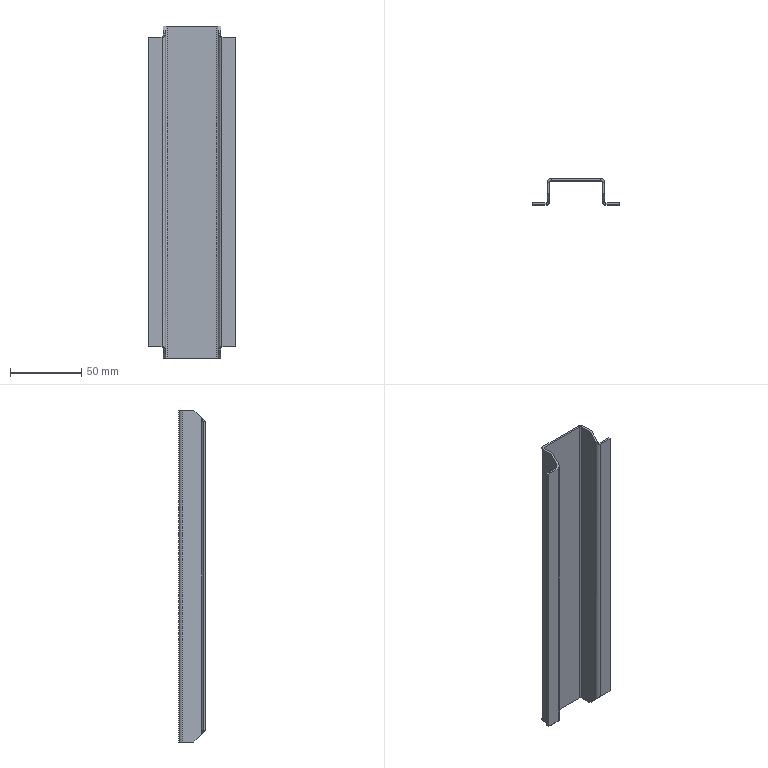Part | SolidWorks | features FlatPattern 1, ICE 1, SMBaseFlange 1, SheetMetal 1 | 1 solid | 42 faces | box 61 x 18.5 x 232.5 mm | volume 31420 mm3 | plane 30 | cylinder 8 | spline 4 | commonest cylinder face diameters 2 x4 5 x4
STEP:
#1=CARTESIAN_POINT('',(22.477,26.708,8.));
#2=VERTEX_POINT('',#1);
#3=CARTESIAN_POINT('',(12.977,26.708,8.));
#4=VERTEX_POINT('',#3);
#5=CARTESIAN_POINT('',(168.477,26.708,8.));
#6=DIRECTION('',(-1.,0.,0.));
#7=VECTOR('',#6,1000.);
#8=LINE('',#5,#7);
#9=EDGE_CURVE('',#2,#4,#8,.T.);
#10=ORIENTED_EDGE('',*,*,#9,.F.);
#11=CARTESIAN_POINT('',(22.477,26.708,224.5));
#12=VERTEX_POINT('',#11);
#13=CARTESIAN_POINT('',(22.477,26.708,232.5));
#14=DIRECTION('',(0.,0.,-1.));
#15=VECTOR('',#14,1000.);
#16=LINE('',#13,#15);
#17=EDGE_CURVE('',#12,#2,#16,.T.);
#18=ORIENTED_EDGE('',*,*,#17,.F.);
#19=CARTESIAN_POINT('',(12.977,26.708,224.5));
#20=VERTEX_POINT('',#19);
#21=CARTESIAN_POINT('',(168.477,26.708,224.5));
#22=DIRECTION('',(-1.,0.,0.));
#23=VECTOR('',#22,1000.);
#24=LINE('',#21,#23);
#25=EDGE_CURVE('',#12,#20,#24,.T.);
#26=ORIENTED_EDGE('',*,*,#25,.T.);
#27=CARTESIAN_POINT('',(12.977,26.708,232.5));
#28=DIRECTION('',(0.,0.,-1.));
#29=VECTOR('',#28,1000.);
#30=LINE('',#27,#29);
#31=EDGE_CURVE('',#20,#4,#30,.T.);
#32=ORIENTED_EDGE('',*,*,#31,.T.);
#33=EDGE_LOOP('',(#10,#18,#26,#32));
#34=FACE_OUTER_BOUND('',#33,.T.);
#35=CARTESIAN_POINT('',(11.977,26.708,232.5));
#36=DIRECTION('',(0.,1.,0.));
#37=DIRECTION('',(-1.,0.,0.));
#38=AXIS2_PLACEMENT_3D('',#35,#36,#37);
#39=PLANE('',#38);
#40=ADVANCED_FACE('',(#34),#39,.F.);
#41=ORIENTED_EDGE('',*,*,#17,.T.);
#42=CARTESIAN_POINT('',(22.477,28.208,8.));
#43=VERTEX_POINT('',#42);
#44=CARTESIAN_POINT('',(22.477,26.708,8.));
#45=DIRECTION('',(0.,1.,0.));
#46=VECTOR('',#45,1000.);
#47=LINE('',#44,#46);
#48=EDGE_CURVE('',#2,#43,#47,.T.);
#49=ORIENTED_EDGE('',*,*,#48,.T.);
#50=CARTESIAN_POINT('',(22.477,28.208,224.5));
#51=VERTEX_POINT('',#50);
#52=CARTESIAN_POINT('',(22.477,28.208,232.5));
#53=DIRECTION('',(0.,0.,-1.));
#54=VECTOR('',#53,1000.);
#55=LINE('',#52,#54);
#56=EDGE_CURVE('',#51,#43,#55,.T.);
#57=ORIENTED_EDGE('',*,*,#56,.F.);
#58=CARTESIAN_POINT('',(22.477,26.708,224.5));
#59=DIRECTION('',(0.,1.,0.));
#60=VECTOR('',#59,1000.);
#61=LINE('',#58,#60);
#62=EDGE_CURVE('',#12,#51,#61,.T.);
#63=ORIENTED_EDGE('',*,*,#62,.F.);
#64=EDGE_LOOP('',(#41,#49,#57,#63));
#65=FACE_OUTER_BOUND('',#64,.T.);
#66=CARTESIAN_POINT('',(22.477,28.208,232.5));
#67=DIRECTION('',(1.,0.,0.));
#68=DIRECTION('',(0.,0.,-1.));
#69=AXIS2_PLACEMENT_3D('',#66,#67,#68);
#70=PLANE('',#69);
#71=ADVANCED_FACE('',(#65),#70,.T.);
#72=ORIENTED_EDGE('',*,*,#56,.T.);
#73=CARTESIAN_POINT('',(12.977,28.208,8.));
#74=VERTEX_POINT('',#73);
#75=CARTESIAN_POINT('',(11.977,28.208,8.));
#76=DIRECTION('',(-1.,0.,0.));
#77=VECTOR('',#76,1000.);
#78=LINE('',#75,#77);
#79=EDGE_CURVE('',#43,#74,#78,.T.);
#80=ORIENTED_EDGE('',*,*,#79,.T.);
#81=CARTESIAN_POINT('',(12.977,28.208,224.5));
#82=VERTEX_POINT('',#81);
#83=CARTESIAN_POINT('',(12.977,28.208,232.5));
#84=DIRECTION('',(0.,0.,-1.));
#85=VECTOR('',#84,1000.);
#86=LINE('',#83,#85);
#87=EDGE_CURVE('',#82,#74,#86,.T.);
#88=ORIENTED_EDGE('',*,*,#87,.F.);
#89=CARTESIAN_POINT('',(11.977,28.208,224.5));
#90=DIRECTION('',(-1.,0.,0.));
#91=VECTOR('',#90,1000.);
#92=LINE('',#89,#91);
#93=EDGE_CURVE('',#51,#82,#92,.T.);
#94=ORIENTED_EDGE('',*,*,#93,.F.);
#95=EDGE_LOOP('',(#72,#80,#88,#94));
#96=FACE_OUTER_BOUND('',#95,.T.);
#97=CARTESIAN_POINT('',(11.977,28.208,232.5));
#98=DIRECTION('',(0.,1.,0.));
#99=DIRECTION('',(-1.,0.,0.));
#100=AXIS2_PLACEMENT_3D('',#97,#98,#99);
#101=PLANE('',#100);
#102=ADVANCED_FACE('',(#96),#101,.T.);
#103=ORIENTED_EDGE('',*,*,#87,.T.);
#104=CARTESIAN_POINT('',(11.977,29.208,5.5));
#105=VERTEX_POINT('',#104);
#106=CARTESIAN_POINT('',(11.977,29.208,5.5));
#107=CARTESIAN_POINT('',(11.977,28.623,6.964));
#108=CARTESIAN_POINT('',(12.391,28.208,8.));
#109=CARTESIAN_POINT('',(12.977,28.208,8.));
#110=(BOUNDED_CURVE()B_SPLINE_CURVE(3,(#106,#107,#108,#109),.UNSPECIFIED.,.F.,.F.)B_SPLINE_CURVE_WITH_KNOTS((4,4),(1.571,3.142),.UNSPECIFIED.)CURVE()GEOMETRIC_REPRESENTATION_ITEM()RATIONAL_B_SPLINE_CURVE((1.,0.8047,0.8047,1.))REPRESENTATION_ITEM(''));
#111=EDGE_CURVE('',#105,#74,#110,.T.);
#112=ORIENTED_EDGE('',*,*,#111,.F.);
#113=CARTESIAN_POINT('',(11.977,29.208,227.));
#114=VERTEX_POINT('',#113);
#115=CARTESIAN_POINT('',(11.977,29.208,232.5));
#116=DIRECTION('',(0.,0.,-1.));
#117=VECTOR('',#116,1000.);
#118=LINE('',#115,#117);
#119=EDGE_CURVE('',#114,#105,#118,.T.);
#120=ORIENTED_EDGE('',*,*,#119,.F.);
#121=CARTESIAN_POINT('',(12.977,28.208,224.5));
#122=CARTESIAN_POINT('',(12.391,28.208,224.5));
#123=CARTESIAN_POINT('',(11.977,28.623,225.536));
#124=CARTESIAN_POINT('',(11.977,29.208,227.));
#125=(BOUNDED_CURVE()B_SPLINE_CURVE(3,(#121,#122,#123,#124),.UNSPECIFIED.,.F.,.F.)B_SPLINE_CURVE_WITH_KNOTS((4,4),(0.,1.571),.UNSPECIFIED.)CURVE()GEOMETRIC_REPRESENTATION_ITEM()RATIONAL_B_SPLINE_CURVE((1.,0.8047,0.8047,1.))REPRESENTATION_ITEM(''));
#126=EDGE_CURVE('',#82,#114,#125,.T.);
#127=ORIENTED_EDGE('',*,*,#126,.F.);
#128=EDGE_LOOP('',(#103,#112,#120,#127));
#129=FACE_OUTER_BOUND('',#128,.T.);
#130=CARTESIAN_POINT('',(12.977,29.208,232.5));
#131=DIRECTION('',(0.,0.,-1.));
#132=DIRECTION('',(-1.,0.,0.));
#133=AXIS2_PLACEMENT_3D('',#130,#131,#132);
#134=CYLINDRICAL_SURFACE('',#133,1.);
#135=ADVANCED_FACE('',(#129),#134,.F.);
#136=ORIENTED_EDGE('',*,*,#119,.T.);
#137=CARTESIAN_POINT('',(11.977,34.708,0.));
#138=VERTEX_POINT('',#137);
#139=CARTESIAN_POINT('',(11.977,-76.292,111.));
#140=DIRECTION('',(0.,-0.7071,0.7071));
#141=VECTOR('',#140,1000.);
#142=LINE('',#139,#141);
#143=EDGE_CURVE('',#138,#105,#142,.T.);
#144=ORIENTED_EDGE('',*,*,#143,.F.);
#145=CARTESIAN_POINT('',(11.977,42.708,0.));
#146=VERTEX_POINT('',#145);
#147=CARTESIAN_POINT('',(11.977,45.208,0.));
#148=DIRECTION('',(0.,-1.,0.));
#149=VECTOR('',#148,1000.);
#150=LINE('',#147,#149);
#151=EDGE_CURVE('',#146,#138,#150,.T.);
#152=ORIENTED_EDGE('',*,*,#151,.F.);
#153=CARTESIAN_POINT('',(11.977,42.708,232.5));
#154=VERTEX_POINT('',#153);
#155=CARTESIAN_POINT('',(11.977,42.708,232.5));
#156=DIRECTION('',(0.,0.,-1.));
#157=VECTOR('',#156,1000.);
#158=LINE('',#155,#157);
#159=EDGE_CURVE('',#154,#146,#158,.T.);
#160=ORIENTED_EDGE('',*,*,#159,.F.);
#161=CARTESIAN_POINT('',(11.977,34.708,232.5));
#162=VERTEX_POINT('',#161);
#163=CARTESIAN_POINT('',(11.977,45.208,232.5));
#164=DIRECTION('',(0.,-1.,0.));
#165=VECTOR('',#164,1000.);
#166=LINE('',#163,#165);
#167=EDGE_CURVE('',#154,#162,#166,.T.);
#168=ORIENTED_EDGE('',*,*,#167,.T.);
#169=CARTESIAN_POINT('',(11.977,39.958,237.75));
#170=DIRECTION('',(0.,0.7071,0.7071));
#171=VECTOR('',#170,1000.);
#172=LINE('',#169,#171);
#173=EDGE_CURVE('',#114,#162,#172,.T.);
#174=ORIENTED_EDGE('',*,*,#173,.F.);
#175=EDGE_LOOP('',(#136,#144,#152,#160,#168,#174));
#176=FACE_OUTER_BOUND('',#175,.T.);
#177=CARTESIAN_POINT('',(11.977,45.208,232.5));
#178=DIRECTION('',(1.,0.,0.));
#179=DIRECTION('',(0.,1.,0.));
#180=AXIS2_PLACEMENT_3D('',#177,#178,#179);
#181=PLANE('',#180);
#182=ADVANCED_FACE('',(#176),#181,.T.);
#183=CARTESIAN_POINT('',(10.477,34.708,0.));
#184=VERTEX_POINT('',#183);
#185=CARTESIAN_POINT('',(10.477,29.208,5.5));
#186=VERTEX_POINT('',#185);
#187=CARTESIAN_POINT('',(10.477,-76.292,111.));
#188=DIRECTION('',(0.,-0.7071,0.7071));
#189=VECTOR('',#188,1000.);
#190=LINE('',#187,#189);
#191=EDGE_CURVE('',#184,#186,#190,.T.);
#192=ORIENTED_EDGE('',*,*,#191,.T.);
#193=CARTESIAN_POINT('',(10.477,29.208,227.));
#194=VERTEX_POINT('',#193);
#195=CARTESIAN_POINT('',(10.477,29.208,232.5));
#196=DIRECTION('',(0.,0.,-1.));
#197=VECTOR('',#196,1000.);
#198=LINE('',#195,#197);
#199=EDGE_CURVE('',#194,#186,#198,.T.);
#200=ORIENTED_EDGE('',*,*,#199,.F.);
#201=CARTESIAN_POINT('',(10.477,34.708,232.5));
#202=VERTEX_POINT('',#201);
#203=CARTESIAN_POINT('',(10.477,39.958,237.75));
#204=DIRECTION('',(0.,0.7071,0.7071));
#205=VECTOR('',#204,1000.);
#206=LINE('',#203,#205);
#207=EDGE_CURVE('',#194,#202,#206,.T.);
#208=ORIENTED_EDGE('',*,*,#207,.T.);
#209=CARTESIAN_POINT('',(10.477,42.708,232.5));
#210=VERTEX_POINT('',#209);
#211=CARTESIAN_POINT('',(10.477,45.208,232.5));
#212=DIRECTION('',(0.,-1.,0.));
#213=VECTOR('',#212,1000.);
#214=LINE('',#211,#213);
#215=EDGE_CURVE('',#210,#202,#214,.T.);
#216=ORIENTED_EDGE('',*,*,#215,.F.);
#217=CARTESIAN_POINT('',(10.477,42.708,0.));
#218=VERTEX_POINT('',#217);
#219=CARTESIAN_POINT('',(10.477,42.708,232.5));
#220=DIRECTION('',(0.,0.,-1.));
#221=VECTOR('',#220,1000.);
#222=LINE('',#219,#221);
#223=EDGE_CURVE('',#210,#218,#222,.T.);
#224=ORIENTED_EDGE('',*,*,#223,.T.);
#225=CARTESIAN_POINT('',(10.477,45.208,0.));
#226=DIRECTION('',(0.,-1.,0.));
#227=VECTOR('',#226,1000.);
#228=LINE('',#225,#227);
#229=EDGE_CURVE('',#218,#184,#228,.T.);
#230=ORIENTED_EDGE('',*,*,#229,.T.);
#231=EDGE_LOOP('',(#192,#200,#208,#216,#224,#230));
#232=FACE_OUTER_BOUND('',#231,.T.);
#233=CARTESIAN_POINT('',(10.477,45.208,232.5));
#234=DIRECTION('',(1.,0.,0.));
#235=DIRECTION('',(0.,1.,0.));
#236=AXIS2_PLACEMENT_3D('',#233,#234,#235);
#237=PLANE('',#236);
#238=ADVANCED_FACE('',(#232),#237,.F.);
#239=CARTESIAN_POINT('',(10.477,29.208,5.5));
#240=CARTESIAN_POINT('',(10.477,27.744,6.964));
#241=CARTESIAN_POINT('',(11.512,26.708,8.));
#242=CARTESIAN_POINT('',(12.977,26.708,8.));
#243=(BOUNDED_CURVE()B_SPLINE_CURVE(3,(#239,#240,#241,#242),.UNSPECIFIED.,.F.,.F.)B_SPLINE_CURVE_WITH_KNOTS((4,4),(1.571,3.142),.UNSPECIFIED.)CURVE()GEOMETRIC_REPRESENTATION_ITEM()RATIONAL_B_SPLINE_CURVE((1.,0.8047,0.8047,1.))REPRESENTATION_ITEM(''));
#244=EDGE_CURVE('',#186,#4,#243,.T.);
#245=ORIENTED_EDGE('',*,*,#244,.T.);
#246=ORIENTED_EDGE('',*,*,#31,.F.);
#247=CARTESIAN_POINT('',(12.977,26.708,224.5));
#248=CARTESIAN_POINT('',(11.512,26.708,224.5));
#249=CARTESIAN_POINT('',(10.477,27.744,225.536));
#250=CARTESIAN_POINT('',(10.477,29.208,227.));
#251=(BOUNDED_CURVE()B_SPLINE_CURVE(3,(#247,#248,#249,#250),.UNSPECIFIED.,.F.,.F.)B_SPLINE_CURVE_WITH_KNOTS((4,4),(0.,1.571),.UNSPECIFIED.)CURVE()GEOMETRIC_REPRESENTATION_ITEM()RATIONAL_B_SPLINE_CURVE((1.,0.8047,0.8047,1.))REPRESENTATION_ITEM(''));
#252=EDGE_CURVE('',#20,#194,#251,.T.);
#253=ORIENTED_EDGE('',*,*,#252,.T.);
#254=ORIENTED_EDGE('',*,*,#199,.T.);
#255=EDGE_LOOP('',(#245,#246,#253,#254));
#256=FACE_OUTER_BOUND('',#255,.T.);
#257=CARTESIAN_POINT('',(12.977,29.208,232.5));
#258=DIRECTION('',(0.,0.,-1.));
#259=DIRECTION('',(-1.,0.,0.));
#260=AXIS2_PLACEMENT_3D('',#257,#258,#259);
#261=CYLINDRICAL_SURFACE('',#260,2.5);
#262=ADVANCED_FACE('',(#256),#261,.T.);
#263=CARTESIAN_POINT('',(-28.023,34.708,0.));
#264=VERTEX_POINT('',#263);
#265=CARTESIAN_POINT('',(-28.023,42.708,0.));
#266=VERTEX_POINT('',#265);
#267=CARTESIAN_POINT('',(-28.023,28.208,0.));
#268=DIRECTION('',(0.,1.,0.));
#269=VECTOR('',#268,1000.);
#270=LINE('',#267,#269);
#271=EDGE_CURVE('',#264,#266,#270,.T.);
#272=ORIENTED_EDGE('',*,*,#271,.F.);
#273=CARTESIAN_POINT('',(-28.023,29.208,5.5));
#274=VERTEX_POINT('',#273);
#275=CARTESIAN_POINT('',(-28.023,-84.792,119.5));
#276=DIRECTION('',(0.,0.7071,-0.7071));
#277=VECTOR('',#276,1000.);
#278=LINE('',#275,#277);
#279=EDGE_CURVE('',#274,#264,#278,.T.);
#280=ORIENTED_EDGE('',*,*,#279,.F.);
#281=CARTESIAN_POINT('',(-28.023,29.208,227.));
#282=VERTEX_POINT('',#281);
#283=CARTESIAN_POINT('',(-28.023,29.208,232.5));
#284=DIRECTION('',(0.,0.,-1.));
#285=VECTOR('',#284,1000.);
#286=LINE('',#283,#285);
#287=EDGE_CURVE('',#282,#274,#286,.T.);
#288=ORIENTED_EDGE('',*,*,#287,.F.);
#289=CARTESIAN_POINT('',(-28.023,34.708,232.5));
#290=VERTEX_POINT('',#289);
#291=CARTESIAN_POINT('',(-28.023,31.458,229.25));
#292=DIRECTION('',(0.,-0.7071,-0.7071));
#293=VECTOR('',#292,1000.);
#294=LINE('',#291,#293);
#295=EDGE_CURVE('',#290,#282,#294,.T.);
#296=ORIENTED_EDGE('',*,*,#295,.F.);
#297=CARTESIAN_POINT('',(-28.023,42.708,232.5));
#298=VERTEX_POINT('',#297);
#299=CARTESIAN_POINT('',(-28.023,28.208,232.5));
#300=DIRECTION('',(0.,1.,0.));
#301=VECTOR('',#300,1000.);
#302=LINE('',#299,#301);
#303=EDGE_CURVE('',#290,#298,#302,.T.);
#304=ORIENTED_EDGE('',*,*,#303,.T.);
#305=CARTESIAN_POINT('',(-28.023,42.708,232.5));
#306=DIRECTION('',(0.,0.,-1.));
#307=VECTOR('',#306,1000.);
#308=LINE('',#305,#307);
#309=EDGE_CURVE('',#298,#266,#308,.T.);
#310=ORIENTED_EDGE('',*,*,#309,.T.);
#311=EDGE_LOOP('',(#272,#280,#288,#296,#304,#310));
#312=FACE_OUTER_BOUND('',#311,.T.);
#313=CARTESIAN_POINT('',(-28.023,28.208,232.5));
#314=DIRECTION('',(-1.,0.,0.));
#315=DIRECTION('',(0.,0.,1.));
#316=AXIS2_PLACEMENT_3D('',#313,#314,#315);
#317=PLANE('',#316);
#318=ADVANCED_FACE('',(#312),#317,.T.);
#319=ORIENTED_EDGE('',*,*,#287,.T.);
#320=CARTESIAN_POINT('',(-29.023,28.208,8.));
#321=VERTEX_POINT('',#320);
#322=CARTESIAN_POINT('',(-29.023,28.208,8.));
#323=CARTESIAN_POINT('',(-28.437,28.208,8.));
#324=CARTESIAN_POINT('',(-28.023,28.623,6.964));
#325=CARTESIAN_POINT('',(-28.023,29.208,5.5));
#326=(BOUNDED_CURVE()B_SPLINE_CURVE(3,(#322,#323,#324,#325),.UNSPECIFIED.,.F.,.F.)B_SPLINE_CURVE_WITH_KNOTS((4,4),(3.142,4.712),.UNSPECIFIED.)CURVE()GEOMETRIC_REPRESENTATION_ITEM()RATIONAL_B_SPLINE_CURVE((1.,0.8047,0.8047,1.))REPRESENTATION_ITEM(''));
#327=EDGE_CURVE('',#321,#274,#326,.T.);
#328=ORIENTED_EDGE('',*,*,#327,.F.);
#329=CARTESIAN_POINT('',(-29.023,28.208,224.5));
#330=VERTEX_POINT('',#329);
#331=CARTESIAN_POINT('',(-29.023,28.208,232.5));
#332=DIRECTION('',(0.,0.,-1.));
#333=VECTOR('',#332,1000.);
#334=LINE('',#331,#333);
#335=EDGE_CURVE('',#330,#321,#334,.T.);
#336=ORIENTED_EDGE('',*,*,#335,.F.);
#337=CARTESIAN_POINT('',(-28.023,29.208,227.));
#338=CARTESIAN_POINT('',(-28.023,28.623,225.536));
#339=CARTESIAN_POINT('',(-28.437,28.208,224.5));
#340=CARTESIAN_POINT('',(-29.023,28.208,224.5));
#341=(BOUNDED_CURVE()B_SPLINE_CURVE(3,(#337,#338,#339,#340),.UNSPECIFIED.,.F.,.F.)B_SPLINE_CURVE_WITH_KNOTS((4,4),(4.712,6.283),.UNSPECIFIED.)CURVE()GEOMETRIC_REPRESENTATION_ITEM()RATIONAL_B_SPLINE_CURVE((1.,0.8047,0.8047,1.))REPRESENTATION_ITEM(''));
#342=EDGE_CURVE('',#282,#330,#341,.T.);
#343=ORIENTED_EDGE('',*,*,#342,.F.);
#344=EDGE_LOOP('',(#319,#328,#336,#343));
#345=FACE_OUTER_BOUND('',#344,.T.);
#346=CARTESIAN_POINT('',(-29.023,29.208,232.5));
#347=DIRECTION('',(0.,0.,-1.));
#348=DIRECTION('',(-1.,0.,0.));
#349=AXIS2_PLACEMENT_3D('',#346,#347,#348);
#350=CYLINDRICAL_SURFACE('',#349,1.);
#351=ADVANCED_FACE('',(#345),#350,.F.);
#352=ORIENTED_EDGE('',*,*,#335,.T.);
#353=CARTESIAN_POINT('',(-38.523,28.208,8.));
#354=VERTEX_POINT('',#353);
#355=CARTESIAN_POINT('',(-38.523,28.208,8.));
#356=DIRECTION('',(-1.,0.,0.));
#357=VECTOR('',#356,1000.);
#358=LINE('',#355,#357);
#359=EDGE_CURVE('',#321,#354,#358,.T.);
#360=ORIENTED_EDGE('',*,*,#359,.T.);
#361=CARTESIAN_POINT('',(-38.523,28.208,224.5));
#362=VERTEX_POINT('',#361);
#363=CARTESIAN_POINT('',(-38.523,28.208,232.5));
#364=DIRECTION('',(0.,0.,-1.));
#365=VECTOR('',#364,1000.);
#366=LINE('',#363,#365);
#367=EDGE_CURVE('',#362,#354,#366,.T.);
#368=ORIENTED_EDGE('',*,*,#367,.F.);
#369=CARTESIAN_POINT('',(-38.523,28.208,224.5));
#370=DIRECTION('',(-1.,0.,0.));
#371=VECTOR('',#370,1000.);
#372=LINE('',#369,#371);
#373=EDGE_CURVE('',#330,#362,#372,.T.);
#374=ORIENTED_EDGE('',*,*,#373,.F.);
#375=EDGE_LOOP('',(#352,#360,#368,#374));
#376=FACE_OUTER_BOUND('',#375,.T.);
#377=CARTESIAN_POINT('',(-38.523,28.208,232.5));
#378=DIRECTION('',(0.,1.,0.));
#379=DIRECTION('',(0.,0.,1.));
#380=AXIS2_PLACEMENT_3D('',#377,#378,#379);
#381=PLANE('',#380);
#382=ADVANCED_FACE('',(#376),#381,.T.);
#383=ORIENTED_EDGE('',*,*,#367,.T.);
#384=CARTESIAN_POINT('',(-38.523,26.708,8.));
#385=VERTEX_POINT('',#384);
#386=CARTESIAN_POINT('',(-38.523,26.708,8.));
#387=DIRECTION('',(0.,1.,0.));
#388=VECTOR('',#387,1000.);
#389=LINE('',#386,#388);
#390=EDGE_CURVE('',#385,#354,#389,.T.);
#391=ORIENTED_EDGE('',*,*,#390,.F.);
#392=CARTESIAN_POINT('',(-38.523,26.708,224.5));
#393=VERTEX_POINT('',#392);
#394=CARTESIAN_POINT('',(-38.523,26.708,232.5));
#395=DIRECTION('',(0.,0.,-1.));
#396=VECTOR('',#395,1000.);
#397=LINE('',#394,#396);
#398=EDGE_CURVE('',#393,#385,#397,.T.);
#399=ORIENTED_EDGE('',*,*,#398,.F.);
#400=CARTESIAN_POINT('',(-38.523,26.708,224.5));
#401=DIRECTION('',(0.,1.,0.));
#402=VECTOR('',#401,1000.);
#403=LINE('',#400,#402);
#404=EDGE_CURVE('',#393,#362,#403,.T.);
#405=ORIENTED_EDGE('',*,*,#404,.T.);
#406=EDGE_LOOP('',(#383,#391,#399,#405));
#407=FACE_OUTER_BOUND('',#406,.T.);
#408=CARTESIAN_POINT('',(-38.523,26.708,232.5));
#409=DIRECTION('',(-1.,0.,0.));
#410=DIRECTION('',(0.,0.,1.));
#411=AXIS2_PLACEMENT_3D('',#408,#409,#410);
#412=PLANE('',#411);
#413=ADVANCED_FACE('',(#407),#412,.T.);
#414=CARTESIAN_POINT('',(-29.023,26.708,8.));
#415=VERTEX_POINT('',#414);
#416=CARTESIAN_POINT('',(168.477,26.708,8.));
#417=DIRECTION('',(-1.,0.,0.));
#418=VECTOR('',#417,1000.);
#419=LINE('',#416,#418);
#420=EDGE_CURVE('',#415,#385,#419,.T.);
#421=ORIENTED_EDGE('',*,*,#420,.F.);
#422=CARTESIAN_POINT('',(-29.023,26.708,224.5));
#423=VERTEX_POINT('',#422);
#424=CARTESIAN_POINT('',(-29.023,26.708,232.5));
#425=DIRECTION('',(0.,0.,-1.));
#426=VECTOR('',#425,1000.);
#427=LINE('',#424,#426);
#428=EDGE_CURVE('',#423,#415,#427,.T.);
#429=ORIENTED_EDGE('',*,*,#428,.F.);
#430=CARTESIAN_POINT('',(168.477,26.708,224.5));
#431=DIRECTION('',(-1.,0.,0.));
#432=VECTOR('',#431,1000.);
#433=LINE('',#430,#432);
#434=EDGE_CURVE('',#423,#393,#433,.T.);
#435=ORIENTED_EDGE('',*,*,#434,.T.);
#436=ORIENTED_EDGE('',*,*,#398,.T.);
#437=EDGE_LOOP('',(#421,#429,#435,#436));
#438=FACE_OUTER_BOUND('',#437,.T.);
#439=CARTESIAN_POINT('',(-38.523,26.708,232.5));
#440=DIRECTION('',(0.,1.,0.));
#441=DIRECTION('',(0.,0.,1.));
#442=AXIS2_PLACEMENT_3D('',#439,#440,#441);
#443=PLANE('',#442);
#444=ADVANCED_FACE('',(#438),#443,.F.);
#445=CARTESIAN_POINT('',(-26.523,29.208,5.5));
#446=VERTEX_POINT('',#445);
#447=CARTESIAN_POINT('',(-29.023,26.708,8.));
#448=CARTESIAN_POINT('',(-27.559,26.708,8.));
#449=CARTESIAN_POINT('',(-26.523,27.744,6.964));
#450=CARTESIAN_POINT('',(-26.523,29.208,5.5));
#451=(BOUNDED_CURVE()B_SPLINE_CURVE(3,(#447,#448,#449,#450),.UNSPECIFIED.,.F.,.F.)B_SPLINE_CURVE_WITH_KNOTS((4,4),(3.142,4.712),.UNSPECIFIED.)CURVE()GEOMETRIC_REPRESENTATION_ITEM()RATIONAL_B_SPLINE_CURVE((1.,0.8047,0.8047,1.))REPRESENTATION_ITEM(''));
#452=EDGE_CURVE('',#415,#446,#451,.T.);
#453=ORIENTED_EDGE('',*,*,#452,.T.);
#454=CARTESIAN_POINT('',(-26.523,29.208,227.));
#455=VERTEX_POINT('',#454);
#456=CARTESIAN_POINT('',(-26.523,29.208,232.5));
#457=DIRECTION('',(0.,0.,-1.));
#458=VECTOR('',#457,1000.);
#459=LINE('',#456,#458);
#460=EDGE_CURVE('',#455,#446,#459,.T.);
#461=ORIENTED_EDGE('',*,*,#460,.F.);
#462=CARTESIAN_POINT('',(-26.523,29.208,227.));
#463=CARTESIAN_POINT('',(-26.523,27.744,225.536));
#464=CARTESIAN_POINT('',(-27.559,26.708,224.5));
#465=CARTESIAN_POINT('',(-29.023,26.708,224.5));
#466=(BOUNDED_CURVE()B_SPLINE_CURVE(3,(#462,#463,#464,#465),.UNSPECIFIED.,.F.,.T.)B_SPLINE_CURVE_WITH_KNOTS((4,4),(4.712,6.283),.UNSPECIFIED.)CURVE()GEOMETRIC_REPRESENTATION_ITEM()RATIONAL_B_SPLINE_CURVE((1.,0.8047,0.8047,1.))REPRESENTATION_ITEM(''));
#467=EDGE_CURVE('',#455,#423,#466,.T.);
#468=ORIENTED_EDGE('',*,*,#467,.T.);
#469=ORIENTED_EDGE('',*,*,#428,.T.);
#470=EDGE_LOOP('',(#453,#461,#468,#469));
#471=FACE_OUTER_BOUND('',#470,.T.);
#472=CARTESIAN_POINT('',(-29.023,29.208,232.5));
#473=DIRECTION('',(0.,0.,-1.));
#474=DIRECTION('',(-1.,0.,0.));
#475=AXIS2_PLACEMENT_3D('',#472,#473,#474);
#476=CYLINDRICAL_SURFACE('',#475,2.5);
#477=ADVANCED_FACE('',(#471),#476,.T.);
#478=CARTESIAN_POINT('',(-26.523,34.708,0.));
#479=VERTEX_POINT('',#478);
#480=CARTESIAN_POINT('',(-26.523,-84.792,119.5));
#481=DIRECTION('',(0.,0.7071,-0.7071));
#482=VECTOR('',#481,1000.);
#483=LINE('',#480,#482);
#484=EDGE_CURVE('',#446,#479,#483,.T.);
#485=ORIENTED_EDGE('',*,*,#484,.T.);
#486=CARTESIAN_POINT('',(-26.523,42.708,0.));
#487=VERTEX_POINT('',#486);
#488=CARTESIAN_POINT('',(-26.523,28.208,0.));
#489=DIRECTION('',(0.,1.,0.));
#490=VECTOR('',#489,1000.);
#491=LINE('',#488,#490);
#492=EDGE_CURVE('',#479,#487,#491,.T.);
#493=ORIENTED_EDGE('',*,*,#492,.T.);
#494=CARTESIAN_POINT('',(-26.523,42.708,232.5));
#495=VERTEX_POINT('',#494);
#496=CARTESIAN_POINT('',(-26.523,42.708,232.5));
#497=DIRECTION('',(0.,0.,-1.));
#498=VECTOR('',#497,1000.);
#499=LINE('',#496,#498);
#500=EDGE_CURVE('',#495,#487,#499,.T.);
#501=ORIENTED_EDGE('',*,*,#500,.F.);
#502=CARTESIAN_POINT('',(-26.523,34.708,232.5));
#503=VERTEX_POINT('',#502);
#504=CARTESIAN_POINT('',(-26.523,28.208,232.5));
#505=DIRECTION('',(0.,1.,0.));
#506=VECTOR('',#505,1000.);
#507=LINE('',#504,#506);
#508=EDGE_CURVE('',#503,#495,#507,.T.);
#509=ORIENTED_EDGE('',*,*,#508,.F.);
#510=CARTESIAN_POINT('',(-26.523,31.458,229.25));
#511=DIRECTION('',(0.,-0.7071,-0.7071));
#512=VECTOR('',#511,1000.);
#513=LINE('',#510,#512);
#514=EDGE_CURVE('',#503,#455,#513,.T.);
#515=ORIENTED_EDGE('',*,*,#514,.T.);
#516=ORIENTED_EDGE('',*,*,#460,.T.);
#517=EDGE_LOOP('',(#485,#493,#501,#509,#515,#516));
#518=FACE_OUTER_BOUND('',#517,.T.);
#519=CARTESIAN_POINT('',(-26.523,28.208,232.5));
#520=DIRECTION('',(-1.,0.,0.));
#521=DIRECTION('',(0.,0.,1.));
#522=AXIS2_PLACEMENT_3D('',#519,#520,#521);
#523=PLANE('',#522);
#524=ADVANCED_FACE('',(#518),#523,.F.);
#525=ORIENTED_EDGE('',*,*,#303,.F.);
#526=CARTESIAN_POINT('',(-28.023,34.708,232.5));
#527=DIRECTION('',(1.,0.,0.));
#528=VECTOR('',#527,1000.);
#529=LINE('',#526,#528);
#530=EDGE_CURVE('',#290,#503,#529,.T.);
#531=ORIENTED_EDGE('',*,*,#530,.T.);
#532=ORIENTED_EDGE('',*,*,#508,.T.);
#533=CARTESIAN_POINT('',(-26.523,42.708,232.5));
#534=DIRECTION('',(-1.,0.,0.));
#535=VECTOR('',#534,1000.);
#536=LINE('',#533,#535);
#537=EDGE_CURVE('',#495,#298,#536,.T.);
#538=ORIENTED_EDGE('',*,*,#537,.T.);
#539=EDGE_LOOP('',(#525,#531,#532,#538));
#540=FACE_OUTER_BOUND('',#539,.T.);
#541=CARTESIAN_POINT('',(-29.023,26.708,232.5));
#542=DIRECTION('',(0.,0.,1.));
#543=DIRECTION('',(1.,0.,0.));
#544=AXIS2_PLACEMENT_3D('',#541,#542,#543);
#545=PLANE('',#544);
#546=ADVANCED_FACE('',(#540),#545,.T.);
#547=CARTESIAN_POINT('',(-25.523,45.208,232.5));
#548=VERTEX_POINT('',#547);
#549=CARTESIAN_POINT('',(-25.523,43.708,232.5));
#550=VERTEX_POINT('',#549);
#551=CARTESIAN_POINT('',(-25.523,45.208,232.5));
#552=DIRECTION('',(0.,-1.,0.));
#553=VECTOR('',#552,1000.);
#554=LINE('',#551,#553);
#555=EDGE_CURVE('',#548,#550,#554,.T.);
#556=ORIENTED_EDGE('',*,*,#555,.F.);
#557=CARTESIAN_POINT('',(-25.523,42.708,232.5));
#558=DIRECTION('',(0.,0.,-1.));
#559=DIRECTION('',(1.,0.,0.));
#560=AXIS2_PLACEMENT_3D('',#557,#558,#559);
#561=CIRCLE('',#560,2.5);
#562=EDGE_CURVE('',#298,#548,#561,.T.);
#563=ORIENTED_EDGE('',*,*,#562,.F.);
#564=ORIENTED_EDGE('',*,*,#537,.F.);
#565=CARTESIAN_POINT('',(-25.523,42.708,232.5));
#566=DIRECTION('',(0.,0.,-1.));
#567=DIRECTION('',(1.,0.,0.));
#568=AXIS2_PLACEMENT_3D('',#565,#566,#567);
#569=CIRCLE('',#568,1.);
#570=EDGE_CURVE('',#495,#550,#569,.T.);
#571=ORIENTED_EDGE('',*,*,#570,.T.);
#572=EDGE_LOOP('',(#556,#563,#564,#571));
#573=FACE_OUTER_BOUND('',#572,.T.);
#574=CARTESIAN_POINT('',(-25.523,45.208,232.5));
#575=DIRECTION('',(0.,0.,1.));
#576=DIRECTION('',(1.,0.,0.));
#577=AXIS2_PLACEMENT_3D('',#574,#575,#576);
#578=PLANE('',#577);
#579=ADVANCED_FACE('',(#573),#578,.T.);
#580=CARTESIAN_POINT('',(9.477,45.208,232.5));
#581=VERTEX_POINT('',#580);
#582=CARTESIAN_POINT('',(-28.023,45.208,232.5));
#583=DIRECTION('',(1.,0.,0.));
#584=VECTOR('',#583,1000.);
#585=LINE('',#582,#584);
#586=EDGE_CURVE('',#548,#581,#585,.T.);
#587=ORIENTED_EDGE('',*,*,#586,.F.);
#588=ORIENTED_EDGE('',*,*,#555,.T.);
#589=CARTESIAN_POINT('',(9.477,43.708,232.5));
#590=VERTEX_POINT('',#589);
#591=CARTESIAN_POINT('',(-28.023,43.708,232.5));
#592=DIRECTION('',(1.,0.,0.));
#593=VECTOR('',#592,1000.);
#594=LINE('',#591,#593);
#595=EDGE_CURVE('',#550,#590,#594,.T.);
#596=ORIENTED_EDGE('',*,*,#595,.T.);
#597=CARTESIAN_POINT('',(9.477,43.708,232.5));
#598=DIRECTION('',(0.,1.,0.));
#599=VECTOR('',#598,1000.);
#600=LINE('',#597,#599);
#601=EDGE_CURVE('',#590,#581,#600,.T.);
#602=ORIENTED_EDGE('',*,*,#601,.T.);
#603=EDGE_LOOP('',(#587,#588,#596,#602));
#604=FACE_OUTER_BOUND('',#603,.T.);
#605=CARTESIAN_POINT('',(-26.523,42.708,232.5));
#606=DIRECTION('',(0.,0.,1.));
#607=DIRECTION('',(1.,0.,0.));
#608=AXIS2_PLACEMENT_3D('',#605,#606,#607);
#609=PLANE('',#608);
#610=ADVANCED_FACE('',(#604),#609,.T.);
#611=CARTESIAN_POINT('',(-28.023,42.708,0.));
#612=DIRECTION('',(1.,0.,0.));
#613=VECTOR('',#612,1000.);
#614=LINE('',#611,#613);
#615=EDGE_CURVE('',#266,#487,#614,.T.);
#616=ORIENTED_EDGE('',*,*,#615,.F.);
#617=CARTESIAN_POINT('',(-25.523,45.208,0.));
#618=VERTEX_POINT('',#617);
#619=CARTESIAN_POINT('',(-25.523,42.708,0.));
#620=DIRECTION('',(0.,0.,-1.));
#621=DIRECTION('',(1.,0.,0.));
#622=AXIS2_PLACEMENT_3D('',#619,#620,#621);
#623=CIRCLE('',#622,2.5);
#624=EDGE_CURVE('',#266,#618,#623,.T.);
#625=ORIENTED_EDGE('',*,*,#624,.T.);
#626=CARTESIAN_POINT('',(-25.523,43.708,0.));
#627=VERTEX_POINT('',#626);
#628=CARTESIAN_POINT('',(-25.523,43.708,0.));
#629=DIRECTION('',(0.,1.,0.));
#630=VECTOR('',#629,1000.);
#631=LINE('',#628,#630);
#632=EDGE_CURVE('',#627,#618,#631,.T.);
#633=ORIENTED_EDGE('',*,*,#632,.F.);
#634=CARTESIAN_POINT('',(-25.523,42.708,0.));
#635=DIRECTION('',(0.,0.,-1.));
#636=DIRECTION('',(1.,0.,0.));
#637=AXIS2_PLACEMENT_3D('',#634,#635,#636);
#638=CIRCLE('',#637,1.);
#639=EDGE_CURVE('',#487,#627,#638,.T.);
#640=ORIENTED_EDGE('',*,*,#639,.F.);
#641=EDGE_LOOP('',(#616,#625,#633,#640));
#642=FACE_OUTER_BOUND('',#641,.T.);
#643=CARTESIAN_POINT('',(-28.023,42.708,0.));
#644=DIRECTION('',(0.,0.,-1.));
#645=DIRECTION('',(-1.,0.,0.));
#646=AXIS2_PLACEMENT_3D('',#643,#644,#645);
#647=PLANE('',#646);
#648=ADVANCED_FACE('',(#642),#647,.T.);
#649=ORIENTED_EDGE('',*,*,#492,.F.);
#650=CARTESIAN_POINT('',(-28.023,34.708,0.));
#651=DIRECTION('',(1.,0.,0.));
#652=VECTOR('',#651,1000.);
#653=LINE('',#650,#652);
#654=EDGE_CURVE('',#264,#479,#653,.T.);
#655=ORIENTED_EDGE('',*,*,#654,.F.);
#656=ORIENTED_EDGE('',*,*,#271,.T.);
#657=ORIENTED_EDGE('',*,*,#615,.T.);
#658=EDGE_LOOP('',(#649,#655,#656,#657));
#659=FACE_OUTER_BOUND('',#658,.T.);
#660=CARTESIAN_POINT('',(-25.523,43.708,0.));
#661=DIRECTION('',(0.,0.,-1.));
#662=DIRECTION('',(-1.,0.,0.));
#663=AXIS2_PLACEMENT_3D('',#660,#661,#662);
#664=PLANE('',#663);
#665=ADVANCED_FACE('',(#659),#664,.T.);
#666=CARTESIAN_POINT('',(11.977,42.708,232.5));
#667=DIRECTION('',(-1.,0.,0.));
#668=VECTOR('',#667,1000.);
#669=LINE('',#666,#668);
#670=EDGE_CURVE('',#154,#210,#669,.T.);
#671=ORIENTED_EDGE('',*,*,#670,.F.);
#672=CARTESIAN_POINT('',(9.477,42.708,232.5));
#673=DIRECTION('',(0.,0.,-1.));
#674=DIRECTION('',(1.,0.,0.));
#675=AXIS2_PLACEMENT_3D('',#672,#673,#674);
#676=CIRCLE('',#675,2.5);
#677=EDGE_CURVE('',#581,#154,#676,.T.);
#678=ORIENTED_EDGE('',*,*,#677,.F.);
#679=ORIENTED_EDGE('',*,*,#601,.F.);
#680=CARTESIAN_POINT('',(9.477,42.708,232.5));
#681=DIRECTION('',(0.,0.,-1.));
#682=DIRECTION('',(1.,0.,0.));
#683=AXIS2_PLACEMENT_3D('',#680,#681,#682);
#684=CIRCLE('',#683,1.);
#685=EDGE_CURVE('',#590,#210,#684,.T.);
#686=ORIENTED_EDGE('',*,*,#685,.T.);
#687=EDGE_LOOP('',(#671,#678,#679,#686));
#688=FACE_OUTER_BOUND('',#687,.T.);
#689=CARTESIAN_POINT('',(11.977,42.708,232.5));
#690=DIRECTION('',(0.,0.,1.));
#691=DIRECTION('',(1.,0.,0.));
#692=AXIS2_PLACEMENT_3D('',#689,#690,#691);
#693=PLANE('',#692);
#694=ADVANCED_FACE('',(#688),#693,.T.);
#695=ORIENTED_EDGE('',*,*,#215,.T.);
#696=CARTESIAN_POINT('',(10.477,34.708,232.5));
#697=DIRECTION('',(1.,0.,0.));
#698=VECTOR('',#697,1000.);
#699=LINE('',#696,#698);
#700=EDGE_CURVE('',#202,#162,#699,.T.);
#701=ORIENTED_EDGE('',*,*,#700,.T.);
#702=ORIENTED_EDGE('',*,*,#167,.F.);
#703=ORIENTED_EDGE('',*,*,#670,.T.);
#704=EDGE_LOOP('',(#695,#701,#702,#703));
#705=FACE_OUTER_BOUND('',#704,.T.);
#706=CARTESIAN_POINT('',(9.477,43.708,232.5));
#707=DIRECTION('',(0.,0.,1.));
#708=DIRECTION('',(1.,0.,0.));
#709=AXIS2_PLACEMENT_3D('',#706,#707,#708);
#710=PLANE('',#709);
#711=ADVANCED_FACE('',(#705),#710,.T.);
#712=CARTESIAN_POINT('',(9.477,45.208,0.));
#713=VERTEX_POINT('',#712);
#714=CARTESIAN_POINT('',(9.477,43.708,0.));
#715=VERTEX_POINT('',#714);
#716=CARTESIAN_POINT('',(9.477,45.208,0.));
#717=DIRECTION('',(0.,-1.,0.));
#718=VECTOR('',#717,1000.);
#719=LINE('',#716,#718);
#720=EDGE_CURVE('',#713,#715,#719,.T.);
#721=ORIENTED_EDGE('',*,*,#720,.F.);
#722=CARTESIAN_POINT('',(9.477,42.708,0.));
#723=DIRECTION('',(0.,0.,-1.));
#724=DIRECTION('',(1.,0.,0.));
#725=AXIS2_PLACEMENT_3D('',#722,#723,#724);
#726=CIRCLE('',#725,2.5);
#727=EDGE_CURVE('',#713,#146,#726,.T.);
#728=ORIENTED_EDGE('',*,*,#727,.T.);
#729=CARTESIAN_POINT('',(10.477,42.708,0.));
#730=DIRECTION('',(1.,0.,0.));
#731=VECTOR('',#730,1000.);
#732=LINE('',#729,#731);
#733=EDGE_CURVE('',#218,#146,#732,.T.);
#734=ORIENTED_EDGE('',*,*,#733,.F.);
#735=CARTESIAN_POINT('',(9.477,42.708,0.));
#736=DIRECTION('',(0.,0.,-1.));
#737=DIRECTION('',(1.,0.,0.));
#738=AXIS2_PLACEMENT_3D('',#735,#736,#737);
#739=CIRCLE('',#738,1.);
#740=EDGE_CURVE('',#715,#218,#739,.T.);
#741=ORIENTED_EDGE('',*,*,#740,.F.);
#742=EDGE_LOOP('',(#721,#728,#734,#741));
#743=FACE_OUTER_BOUND('',#742,.T.);
#744=CARTESIAN_POINT('',(9.477,45.208,0.));
#745=DIRECTION('',(0.,0.,-1.));
#746=DIRECTION('',(-1.,0.,0.));
#747=AXIS2_PLACEMENT_3D('',#744,#745,#746);
#748=PLANE('',#747);
#749=ADVANCED_FACE('',(#743),#748,.T.);
#750=CARTESIAN_POINT('',(-28.023,45.208,0.));
#751=DIRECTION('',(1.,0.,0.));
#752=VECTOR('',#751,1000.);
#753=LINE('',#750,#752);
#754=EDGE_CURVE('',#618,#713,#753,.T.);
#755=ORIENTED_EDGE('',*,*,#754,.T.);
#756=ORIENTED_EDGE('',*,*,#720,.T.);
#757=CARTESIAN_POINT('',(-28.023,43.708,0.));
#758=DIRECTION('',(1.,0.,0.));
#759=VECTOR('',#758,1000.);
#760=LINE('',#757,#759);
#761=EDGE_CURVE('',#627,#715,#760,.T.);
#762=ORIENTED_EDGE('',*,*,#761,.F.);
#763=ORIENTED_EDGE('',*,*,#632,.T.);
#764=EDGE_LOOP('',(#755,#756,#762,#763));
#765=FACE_OUTER_BOUND('',#764,.T.);
#766=CARTESIAN_POINT('',(10.477,42.708,0.));
#767=DIRECTION('',(0.,0.,-1.));
#768=DIRECTION('',(-1.,0.,0.));
#769=AXIS2_PLACEMENT_3D('',#766,#767,#768);
#770=PLANE('',#769);
#771=ADVANCED_FACE('',(#765),#770,.T.);
#772=ORIENTED_EDGE('',*,*,#151,.T.);
#773=CARTESIAN_POINT('',(11.977,34.708,0.));
#774=DIRECTION('',(-1.,0.,0.));
#775=VECTOR('',#774,1000.);
#776=LINE('',#773,#775);
#777=EDGE_CURVE('',#138,#184,#776,.T.);
#778=ORIENTED_EDGE('',*,*,#777,.T.);
#779=ORIENTED_EDGE('',*,*,#229,.F.);
#780=ORIENTED_EDGE('',*,*,#733,.T.);
#781=EDGE_LOOP('',(#772,#778,#779,#780));
#782=FACE_OUTER_BOUND('',#781,.T.);
#783=CARTESIAN_POINT('',(12.977,26.708,0.));
#784=DIRECTION('',(0.,0.,-1.));
#785=DIRECTION('',(-1.,0.,0.));
#786=AXIS2_PLACEMENT_3D('',#783,#784,#785);
#787=PLANE('',#786);
#788=ADVANCED_FACE('',(#782),#787,.T.);
#789=ORIENTED_EDGE('',*,*,#727,.F.);
#790=CARTESIAN_POINT('',(9.477,45.208,232.5));
#791=DIRECTION('',(0.,0.,-1.));
#792=VECTOR('',#791,1000.);
#793=LINE('',#790,#792);
#794=EDGE_CURVE('',#581,#713,#793,.T.);
#795=ORIENTED_EDGE('',*,*,#794,.F.);
#796=ORIENTED_EDGE('',*,*,#677,.T.);
#797=ORIENTED_EDGE('',*,*,#159,.T.);
#798=EDGE_LOOP('',(#789,#795,#796,#797));
#799=FACE_OUTER_BOUND('',#798,.T.);
#800=CARTESIAN_POINT('',(9.477,42.708,232.5));
#801=DIRECTION('',(0.,0.,-1.));
#802=DIRECTION('',(-1.,0.,0.));
#803=AXIS2_PLACEMENT_3D('',#800,#801,#802);
#804=CYLINDRICAL_SURFACE('',#803,2.5);
#805=ADVANCED_FACE('',(#799),#804,.T.);
#806=ORIENTED_EDGE('',*,*,#754,.F.);
#807=CARTESIAN_POINT('',(-25.523,45.208,232.5));
#808=DIRECTION('',(0.,0.,-1.));
#809=VECTOR('',#808,1000.);
#810=LINE('',#807,#809);
#811=EDGE_CURVE('',#548,#618,#810,.T.);
#812=ORIENTED_EDGE('',*,*,#811,.F.);
#813=ORIENTED_EDGE('',*,*,#586,.T.);
#814=ORIENTED_EDGE('',*,*,#794,.T.);
#815=EDGE_LOOP('',(#806,#812,#813,#814));
#816=FACE_OUTER_BOUND('',#815,.T.);
#817=CARTESIAN_POINT('',(-28.023,45.208,232.5));
#818=DIRECTION('',(0.,1.,0.));
#819=DIRECTION('',(0.,0.,1.));
#820=AXIS2_PLACEMENT_3D('',#817,#818,#819);
#821=PLANE('',#820);
#822=ADVANCED_FACE('',(#816),#821,.T.);
#823=ORIENTED_EDGE('',*,*,#624,.F.);
#824=ORIENTED_EDGE('',*,*,#309,.F.);
#825=ORIENTED_EDGE('',*,*,#562,.T.);
#826=ORIENTED_EDGE('',*,*,#811,.T.);
#827=EDGE_LOOP('',(#823,#824,#825,#826));
#828=FACE_OUTER_BOUND('',#827,.T.);
#829=CARTESIAN_POINT('',(-25.523,42.708,232.5));
#830=DIRECTION('',(0.,0.,-1.));
#831=DIRECTION('',(-1.,0.,0.));
#832=AXIS2_PLACEMENT_3D('',#829,#830,#831);
#833=CYLINDRICAL_SURFACE('',#832,2.5);
#834=ADVANCED_FACE('',(#828),#833,.T.);
#835=ORIENTED_EDGE('',*,*,#639,.T.);
#836=CARTESIAN_POINT('',(-25.523,43.708,232.5));
#837=DIRECTION('',(0.,0.,-1.));
#838=VECTOR('',#837,1000.);
#839=LINE('',#836,#838);
#840=EDGE_CURVE('',#550,#627,#839,.T.);
#841=ORIENTED_EDGE('',*,*,#840,.F.);
#842=ORIENTED_EDGE('',*,*,#570,.F.);
#843=ORIENTED_EDGE('',*,*,#500,.T.);
#844=EDGE_LOOP('',(#835,#841,#842,#843));
#845=FACE_OUTER_BOUND('',#844,.T.);
#846=CARTESIAN_POINT('',(-25.523,42.708,232.5));
#847=DIRECTION('',(0.,0.,-1.));
#848=DIRECTION('',(-1.,0.,0.));
#849=AXIS2_PLACEMENT_3D('',#846,#847,#848);
#850=CYLINDRICAL_SURFACE('',#849,1.);
#851=ADVANCED_FACE('',(#845),#850,.F.);
#852=ORIENTED_EDGE('',*,*,#761,.T.);
#853=CARTESIAN_POINT('',(9.477,43.708,232.5));
#854=DIRECTION('',(0.,0.,-1.));
#855=VECTOR('',#854,1000.);
#856=LINE('',#853,#855);
#857=EDGE_CURVE('',#590,#715,#856,.T.);
#858=ORIENTED_EDGE('',*,*,#857,.F.);
#859=ORIENTED_EDGE('',*,*,#595,.F.);
#860=ORIENTED_EDGE('',*,*,#840,.T.);
#861=EDGE_LOOP('',(#852,#858,#859,#860));
#862=FACE_OUTER_BOUND('',#861,.T.);
#863=CARTESIAN_POINT('',(-28.023,43.708,232.5));
#864=DIRECTION('',(0.,1.,0.));
#865=DIRECTION('',(0.,0.,1.));
#866=AXIS2_PLACEMENT_3D('',#863,#864,#865);
#867=PLANE('',#866);
#868=ADVANCED_FACE('',(#862),#867,.F.);
#869=ORIENTED_EDGE('',*,*,#740,.T.);
#870=ORIENTED_EDGE('',*,*,#223,.F.);
#871=ORIENTED_EDGE('',*,*,#685,.F.);
#872=ORIENTED_EDGE('',*,*,#857,.T.);
#873=EDGE_LOOP('',(#869,#870,#871,#872));
#874=FACE_OUTER_BOUND('',#873,.T.);
#875=CARTESIAN_POINT('',(9.477,42.708,232.5));
#876=DIRECTION('',(0.,0.,-1.));
#877=DIRECTION('',(-1.,0.,0.));
#878=AXIS2_PLACEMENT_3D('',#875,#876,#877);
#879=CYLINDRICAL_SURFACE('',#878,1.);
#880=ADVANCED_FACE('',(#874),#879,.F.);
#881=ORIENTED_EDGE('',*,*,#295,.T.);
#882=CARTESIAN_POINT('',(-28.023,29.208,227.));
#883=DIRECTION('',(1.,0.,0.));
#884=VECTOR('',#883,1000.);
#885=LINE('',#882,#884);
#886=EDGE_CURVE('',#282,#455,#885,.T.);
#887=ORIENTED_EDGE('',*,*,#886,.T.);
#888=ORIENTED_EDGE('',*,*,#514,.F.);
#889=ORIENTED_EDGE('',*,*,#530,.F.);
#890=EDGE_LOOP('',(#881,#887,#888,#889));
#891=FACE_OUTER_BOUND('',#890,.T.);
#892=CARTESIAN_POINT('',(-28.023,31.458,229.25));
#893=DIRECTION('',(0.,0.7071,-0.7071));
#894=DIRECTION('',(0.,-0.7071,-0.7071));
#895=AXIS2_PLACEMENT_3D('',#892,#893,#894);
#896=PLANE('',#895);
#897=ADVANCED_FACE('',(#891),#896,.F.);
#898=ORIENTED_EDGE('',*,*,#404,.F.);
#899=ORIENTED_EDGE('',*,*,#434,.F.);
#900=CARTESIAN_POINT('',(-29.023,26.708,224.5));
#901=DIRECTION('',(0.,1.,0.));
#902=VECTOR('',#901,1000.);
#903=LINE('',#900,#902);
#904=EDGE_CURVE('',#423,#330,#903,.T.);
#905=ORIENTED_EDGE('',*,*,#904,.T.);
#906=ORIENTED_EDGE('',*,*,#373,.T.);
#907=EDGE_LOOP('',(#898,#899,#905,#906));
#908=FACE_OUTER_BOUND('',#907,.T.);
#909=CARTESIAN_POINT('',(168.477,26.708,224.5));
#910=DIRECTION('',(0.,0.,-1.));
#911=DIRECTION('',(-1.,0.,0.));
#912=AXIS2_PLACEMENT_3D('',#909,#910,#911);
#913=PLANE('',#912);
#914=ADVANCED_FACE('',(#908),#913,.F.);
#915=ORIENTED_EDGE('',*,*,#904,.F.);
#916=ORIENTED_EDGE('',*,*,#467,.F.);
#917=ORIENTED_EDGE('',*,*,#886,.F.);
#918=ORIENTED_EDGE('',*,*,#342,.T.);
#919=EDGE_LOOP('',(#915,#916,#917,#918));
#920=FACE_OUTER_BOUND('',#919,.T.);
#921=CARTESIAN_POINT('',(-29.023,28.208,224.5));
#922=CARTESIAN_POINT('',(-29.023,27.708,224.5));
#923=CARTESIAN_POINT('',(-29.023,27.208,224.5));
#924=CARTESIAN_POINT('',(-29.023,26.708,224.5));
#925=CARTESIAN_POINT('',(-31.023,28.208,224.5));
#926=CARTESIAN_POINT('',(-32.023,27.708,224.5));
#927=CARTESIAN_POINT('',(-33.023,27.208,224.5));
#928=CARTESIAN_POINT('',(-34.023,26.708,224.5));
#929=CARTESIAN_POINT('',(-31.023,30.208,229.5));
#930=CARTESIAN_POINT('',(-32.023,30.708,229.5));
#931=CARTESIAN_POINT('',(-33.023,31.208,229.5));
#932=CARTESIAN_POINT('',(-34.023,31.708,229.5));
#933=CARTESIAN_POINT('',(-29.023,30.208,229.5));
#934=CARTESIAN_POINT('',(-29.023,30.708,229.5));
#935=CARTESIAN_POINT('',(-29.023,31.208,229.5));
#936=CARTESIAN_POINT('',(-29.023,31.708,229.5));
#937=CARTESIAN_POINT('',(-27.023,30.208,229.5));
#938=CARTESIAN_POINT('',(-26.023,30.708,229.5));
#939=CARTESIAN_POINT('',(-25.023,31.208,229.5));
#940=CARTESIAN_POINT('',(-24.023,31.708,229.5));
#941=CARTESIAN_POINT('',(-27.023,28.208,224.5));
#942=CARTESIAN_POINT('',(-26.023,27.708,224.5));
#943=CARTESIAN_POINT('',(-25.023,27.208,224.5));
#944=CARTESIAN_POINT('',(-24.023,26.708,224.5));
#945=CARTESIAN_POINT('',(-29.023,28.208,224.5));
#946=CARTESIAN_POINT('',(-29.023,27.708,224.5));
#947=CARTESIAN_POINT('',(-29.023,27.208,224.5));
#948=CARTESIAN_POINT('',(-29.023,26.708,224.5));
#949=(BOUNDED_SURFACE()B_SPLINE_SURFACE(3,3,((#921,#922,#923,#924),(#925,#926,#927,#928),(#929,#930,#931,#932),(#933,#934,#935,#936),(#937,#938,#939,#940),(#941,#942,#943,#944),(#945,#946,#947,#948)),.UNSPECIFIED.,.T.,.F.,.F.)B_SPLINE_SURFACE_WITH_KNOTS((4,3,4),(4,4),(0.,0.5,1.),(0.,1.),.UNSPECIFIED.)GEOMETRIC_REPRESENTATION_ITEM()RATIONAL_B_SPLINE_SURFACE(((1.,1.,1.,1.),(0.3333,0.3333,0.3333,0.3333),(0.3333,0.3333,0.3333,0.3333),(1.,1.,1.,1.),(0.3333,0.3333,0.3333,0.3333),(0.3333,0.3333,0.3333,0.3333),(1.,1.,1.,1.)))REPRESENTATION_ITEM('')SURFACE());
#950=ADVANCED_FACE('',(#920),#949,.T.);
#951=ORIENTED_EDGE('',*,*,#279,.T.);
#952=ORIENTED_EDGE('',*,*,#654,.T.);
#953=ORIENTED_EDGE('',*,*,#484,.F.);
#954=CARTESIAN_POINT('',(-28.023,29.208,5.5));
#955=DIRECTION('',(1.,0.,0.));
#956=VECTOR('',#955,1000.);
#957=LINE('',#954,#956);
#958=EDGE_CURVE('',#274,#446,#957,.T.);
#959=ORIENTED_EDGE('',*,*,#958,.F.);
#960=EDGE_LOOP('',(#951,#952,#953,#959));
#961=FACE_OUTER_BOUND('',#960,.T.);
#962=CARTESIAN_POINT('',(-28.023,-84.792,119.5));
#963=DIRECTION('',(0.,0.7071,0.7071));
#964=DIRECTION('',(0.,0.7071,-0.7071));
#965=AXIS2_PLACEMENT_3D('',#962,#963,#964);
#966=PLANE('',#965);
#967=ADVANCED_FACE('',(#961),#966,.F.);
#968=CARTESIAN_POINT('',(-29.023,26.708,8.));
#969=DIRECTION('',(0.,1.,0.));
#970=VECTOR('',#969,1000.);
#971=LINE('',#968,#970);
#972=EDGE_CURVE('',#415,#321,#971,.T.);
#973=ORIENTED_EDGE('',*,*,#972,.F.);
#974=ORIENTED_EDGE('',*,*,#420,.T.);
#975=ORIENTED_EDGE('',*,*,#390,.T.);
#976=ORIENTED_EDGE('',*,*,#359,.F.);
#977=EDGE_LOOP('',(#973,#974,#975,#976));
#978=FACE_OUTER_BOUND('',#977,.T.);
#979=CARTESIAN_POINT('',(168.477,26.708,8.));
#980=DIRECTION('',(0.,0.,-1.));
#981=DIRECTION('',(-1.,0.,0.));
#982=AXIS2_PLACEMENT_3D('',#979,#980,#981);
#983=PLANE('',#982);
#984=ADVANCED_FACE('',(#978),#983,.T.);
#985=ORIENTED_EDGE('',*,*,#958,.T.);
#986=ORIENTED_EDGE('',*,*,#452,.F.);
#987=ORIENTED_EDGE('',*,*,#972,.T.);
#988=ORIENTED_EDGE('',*,*,#327,.T.);
#989=EDGE_LOOP('',(#985,#986,#987,#988));
#990=FACE_OUTER_BOUND('',#989,.T.);
#991=CARTESIAN_POINT('',(-29.023,30.208,3.));
#992=CARTESIAN_POINT('',(-29.023,30.708,3.));
#993=CARTESIAN_POINT('',(-29.023,31.208,3.));
#994=CARTESIAN_POINT('',(-29.023,31.708,3.));
#995=CARTESIAN_POINT('',(-31.023,30.208,3.));
#996=CARTESIAN_POINT('',(-32.023,30.708,3.));
#997=CARTESIAN_POINT('',(-33.023,31.208,3.));
#998=CARTESIAN_POINT('',(-34.023,31.708,3.));
#999=CARTESIAN_POINT('',(-31.023,28.208,8.));
#1000=CARTESIAN_POINT('',(-32.023,27.708,8.));
#1001=CARTESIAN_POINT('',(-33.023,27.208,8.));
#1002=CARTESIAN_POINT('',(-34.023,26.708,8.));
#1003=CARTESIAN_POINT('',(-29.023,28.208,8.));
#1004=CARTESIAN_POINT('',(-29.023,27.708,8.));
#1005=CARTESIAN_POINT('',(-29.023,27.208,8.));
#1006=CARTESIAN_POINT('',(-29.023,26.708,8.));
#1007=CARTESIAN_POINT('',(-27.023,28.208,8.));
#1008=CARTESIAN_POINT('',(-26.023,27.708,8.));
#1009=CARTESIAN_POINT('',(-25.023,27.208,8.));
#1010=CARTESIAN_POINT('',(-24.023,26.708,8.));
#1011=CARTESIAN_POINT('',(-27.023,30.208,3.));
#1012=CARTESIAN_POINT('',(-26.023,30.708,3.));
#1013=CARTESIAN_POINT('',(-25.023,31.208,3.));
#1014=CARTESIAN_POINT('',(-24.023,31.708,3.));
#1015=CARTESIAN_POINT('',(-29.023,30.208,3.));
#1016=CARTESIAN_POINT('',(-29.023,30.708,3.));
#1017=CARTESIAN_POINT('',(-29.023,31.208,3.));
#1018=CARTESIAN_POINT('',(-29.023,31.708,3.));
#1019=(BOUNDED_SURFACE()B_SPLINE_SURFACE(3,3,((#991,#992,#993,#994),(#995,#996,#997,#998),(#999,#1000,#1001,#1002),(#1003,#1004,#1005,#1006),(#1007,#1008,#1009,#1010),(#1011,#1012,#1013,#1014),(#1015,#1016,#1017,#1018)),.UNSPECIFIED.,.T.,.F.,.F.)B_SPLINE_SURFACE_WITH_KNOTS((4,3,4),(4,4),(0.,0.5,1.),(0.,1.),.UNSPECIFIED.)GEOMETRIC_REPRESENTATION_ITEM()RATIONAL_B_SPLINE_SURFACE(((1.,1.,1.,1.),(0.3333,0.3333,0.3333,0.3333),(0.3333,0.3333,0.3333,0.3333),(1.,1.,1.,1.),(0.3333,0.3333,0.3333,0.3333),(0.3333,0.3333,0.3333,0.3333),(1.,1.,1.,1.)))REPRESENTATION_ITEM('')SURFACE());
#1020=ADVANCED_FACE('',(#990),#1019,.T.);
#1021=CARTESIAN_POINT('',(12.977,26.708,224.5));
#1022=DIRECTION('',(0.,1.,0.));
#1023=VECTOR('',#1022,1000.);
#1024=LINE('',#1021,#1023);
#1025=EDGE_CURVE('',#20,#82,#1024,.T.);
#1026=ORIENTED_EDGE('',*,*,#1025,.F.);
#1027=ORIENTED_EDGE('',*,*,#25,.F.);
#1028=ORIENTED_EDGE('',*,*,#62,.T.);
#1029=ORIENTED_EDGE('',*,*,#93,.T.);
#1030=EDGE_LOOP('',(#1026,#1027,#1028,#1029));
#1031=FACE_OUTER_BOUND('',#1030,.T.);
#1032=CARTESIAN_POINT('',(168.477,26.708,224.5));
#1033=DIRECTION('',(0.,0.,-1.));
#1034=DIRECTION('',(-1.,0.,0.));
#1035=AXIS2_PLACEMENT_3D('',#1032,#1033,#1034);
#1036=PLANE('',#1035);
#1037=ADVANCED_FACE('',(#1031),#1036,.F.);
#1038=ORIENTED_EDGE('',*,*,#700,.F.);
#1039=ORIENTED_EDGE('',*,*,#207,.F.);
#1040=CARTESIAN_POINT('',(10.477,29.208,227.));
#1041=DIRECTION('',(1.,0.,0.));
#1042=VECTOR('',#1041,1000.);
#1043=LINE('',#1040,#1042);
#1044=EDGE_CURVE('',#194,#114,#1043,.T.);
#1045=ORIENTED_EDGE('',*,*,#1044,.T.);
#1046=ORIENTED_EDGE('',*,*,#173,.T.);
#1047=EDGE_LOOP('',(#1038,#1039,#1045,#1046));
#1048=FACE_OUTER_BOUND('',#1047,.T.);
#1049=CARTESIAN_POINT('',(10.477,39.958,237.75));
#1050=DIRECTION('',(0.,0.7071,-0.7071));
#1051=DIRECTION('',(0.,0.7071,0.7071));
#1052=AXIS2_PLACEMENT_3D('',#1049,#1050,#1051);
#1053=PLANE('',#1052);
#1054=ADVANCED_FACE('',(#1048),#1053,.F.);
#1055=ORIENTED_EDGE('',*,*,#1044,.F.);
#1056=ORIENTED_EDGE('',*,*,#252,.F.);
#1057=ORIENTED_EDGE('',*,*,#1025,.T.);
#1058=ORIENTED_EDGE('',*,*,#126,.T.);
#1059=EDGE_LOOP('',(#1055,#1056,#1057,#1058));
#1060=FACE_OUTER_BOUND('',#1059,.T.);
#1061=CARTESIAN_POINT('',(12.977,28.208,224.5));
#1062=CARTESIAN_POINT('',(12.977,27.708,224.5));
#1063=CARTESIAN_POINT('',(12.977,27.208,224.5));
#1064=CARTESIAN_POINT('',(12.977,26.708,224.5));
#1065=CARTESIAN_POINT('',(10.977,28.208,224.5));
#1066=CARTESIAN_POINT('',(9.977,27.708,224.5));
#1067=CARTESIAN_POINT('',(8.977,27.208,224.5));
#1068=CARTESIAN_POINT('',(7.977,26.708,224.5));
#1069=CARTESIAN_POINT('',(10.977,30.208,229.5));
#1070=CARTESIAN_POINT('',(9.977,30.708,229.5));
#1071=CARTESIAN_POINT('',(8.977,31.208,229.5));
#1072=CARTESIAN_POINT('',(7.977,31.708,229.5));
#1073=CARTESIAN_POINT('',(12.977,30.208,229.5));
#1074=CARTESIAN_POINT('',(12.977,30.708,229.5));
#1075=CARTESIAN_POINT('',(12.977,31.208,229.5));
#1076=CARTESIAN_POINT('',(12.977,31.708,229.5));
#1077=CARTESIAN_POINT('',(14.977,30.208,229.5));
#1078=CARTESIAN_POINT('',(15.977,30.708,229.5));
#1079=CARTESIAN_POINT('',(16.977,31.208,229.5));
#1080=CARTESIAN_POINT('',(17.977,31.708,229.5));
#1081=CARTESIAN_POINT('',(14.977,28.208,224.5));
#1082=CARTESIAN_POINT('',(15.977,27.708,224.5));
#1083=CARTESIAN_POINT('',(16.977,27.208,224.5));
#1084=CARTESIAN_POINT('',(17.977,26.708,224.5));
#1085=CARTESIAN_POINT('',(12.977,28.208,224.5));
#1086=CARTESIAN_POINT('',(12.977,27.708,224.5));
#1087=CARTESIAN_POINT('',(12.977,27.208,224.5));
#1088=CARTESIAN_POINT('',(12.977,26.708,224.5));
#1089=(BOUNDED_SURFACE()B_SPLINE_SURFACE(3,3,((#1061,#1062,#1063,#1064),(#1065,#1066,#1067,#1068),(#1069,#1070,#1071,#1072),(#1073,#1074,#1075,#1076),(#1077,#1078,#1079,#1080),(#1081,#1082,#1083,#1084),(#1085,#1086,#1087,#1088)),.UNSPECIFIED.,.T.,.F.,.F.)B_SPLINE_SURFACE_WITH_KNOTS((4,3,4),(4,4),(0.,0.5,1.),(0.,1.),.UNSPECIFIED.)GEOMETRIC_REPRESENTATION_ITEM()RATIONAL_B_SPLINE_SURFACE(((1.,1.,1.,1.),(0.3333,0.3333,0.3333,0.3333),(0.3333,0.3333,0.3333,0.3333),(1.,1.,1.,1.),(0.3333,0.3333,0.3333,0.3333),(0.3333,0.3333,0.3333,0.3333),(1.,1.,1.,1.)))REPRESENTATION_ITEM('')SURFACE());
#1090=ADVANCED_FACE('',(#1060),#1089,.T.);
#1091=ORIENTED_EDGE('',*,*,#48,.F.);
#1092=ORIENTED_EDGE('',*,*,#9,.T.);
#1093=CARTESIAN_POINT('',(12.977,26.708,8.));
#1094=DIRECTION('',(0.,1.,0.));
#1095=VECTOR('',#1094,1000.);
#1096=LINE('',#1093,#1095);
#1097=EDGE_CURVE('',#4,#74,#1096,.T.);
#1098=ORIENTED_EDGE('',*,*,#1097,.T.);
#1099=ORIENTED_EDGE('',*,*,#79,.F.);
#1100=EDGE_LOOP('',(#1091,#1092,#1098,#1099));
#1101=FACE_OUTER_BOUND('',#1100,.T.);
#1102=CARTESIAN_POINT('',(168.477,26.708,8.));
#1103=DIRECTION('',(0.,0.,-1.));
#1104=DIRECTION('',(-1.,0.,0.));
#1105=AXIS2_PLACEMENT_3D('',#1102,#1103,#1104);
#1106=PLANE('',#1105);
#1107=ADVANCED_FACE('',(#1101),#1106,.T.);
#1108=ORIENTED_EDGE('',*,*,#143,.T.);
#1109=CARTESIAN_POINT('',(11.977,29.208,5.5));
#1110=DIRECTION('',(-1.,0.,0.));
#1111=VECTOR('',#1110,1000.);
#1112=LINE('',#1109,#1111);
#1113=EDGE_CURVE('',#105,#186,#1112,.T.);
#1114=ORIENTED_EDGE('',*,*,#1113,.T.);
#1115=ORIENTED_EDGE('',*,*,#191,.F.);
#1116=ORIENTED_EDGE('',*,*,#777,.F.);
#1117=EDGE_LOOP('',(#1108,#1114,#1115,#1116));
#1118=FACE_OUTER_BOUND('',#1117,.T.);
#1119=CARTESIAN_POINT('',(11.977,-76.292,111.));
#1120=DIRECTION('',(0.,0.7071,0.7071));
#1121=DIRECTION('',(0.,-0.7071,0.7071));
#1122=AXIS2_PLACEMENT_3D('',#1119,#1120,#1121);
#1123=PLANE('',#1122);
#1124=ADVANCED_FACE('',(#1118),#1123,.F.);
#1125=ORIENTED_EDGE('',*,*,#1097,.F.);
#1126=ORIENTED_EDGE('',*,*,#244,.F.);
#1127=ORIENTED_EDGE('',*,*,#1113,.F.);
#1128=ORIENTED_EDGE('',*,*,#111,.T.);
#1129=EDGE_LOOP('',(#1125,#1126,#1127,#1128));
#1130=FACE_OUTER_BOUND('',#1129,.T.);
#1131=CARTESIAN_POINT('',(12.977,30.208,3.));
#1132=CARTESIAN_POINT('',(12.977,30.708,3.));
#1133=CARTESIAN_POINT('',(12.977,31.208,3.));
#1134=CARTESIAN_POINT('',(12.977,31.708,3.));
#1135=CARTESIAN_POINT('',(10.977,30.208,3.));
#1136=CARTESIAN_POINT('',(9.977,30.708,3.));
#1137=CARTESIAN_POINT('',(8.977,31.208,3.));
#1138=CARTESIAN_POINT('',(7.977,31.708,3.));
#1139=CARTESIAN_POINT('',(10.977,28.208,8.));
#1140=CARTESIAN_POINT('',(9.977,27.708,8.));
#1141=CARTESIAN_POINT('',(8.977,27.208,8.));
#1142=CARTESIAN_POINT('',(7.977,26.708,8.));
#1143=CARTESIAN_POINT('',(12.977,28.208,8.));
#1144=CARTESIAN_POINT('',(12.977,27.708,8.));
#1145=CARTESIAN_POINT('',(12.977,27.208,8.));
#1146=CARTESIAN_POINT('',(12.977,26.708,8.));
#1147=CARTESIAN_POINT('',(14.977,28.208,8.));
#1148=CARTESIAN_POINT('',(15.977,27.708,8.));
#1149=CARTESIAN_POINT('',(16.977,27.208,8.));
#1150=CARTESIAN_POINT('',(17.977,26.708,8.));
#1151=CARTESIAN_POINT('',(14.977,30.208,3.));
#1152=CARTESIAN_POINT('',(15.977,30.708,3.));
#1153=CARTESIAN_POINT('',(16.977,31.208,3.));
#1154=CARTESIAN_POINT('',(17.977,31.708,3.));
#1155=CARTESIAN_POINT('',(12.977,30.208,3.));
#1156=CARTESIAN_POINT('',(12.977,30.708,3.));
#1157=CARTESIAN_POINT('',(12.977,31.208,3.));
#1158=CARTESIAN_POINT('',(12.977,31.708,3.));
#1159=(BOUNDED_SURFACE()B_SPLINE_SURFACE(3,3,((#1131,#1132,#1133,#1134),(#1135,#1136,#1137,#1138),(#1139,#1140,#1141,#1142),(#1143,#1144,#1145,#1146),(#1147,#1148,#1149,#1150),(#1151,#1152,#1153,#1154),(#1155,#1156,#1157,#1158)),.UNSPECIFIED.,.T.,.F.,.F.)B_SPLINE_SURFACE_WITH_KNOTS((4,3,4),(4,4),(0.,0.5,1.),(0.,1.),.UNSPECIFIED.)GEOMETRIC_REPRESENTATION_ITEM()RATIONAL_B_SPLINE_SURFACE(((1.,1.,1.,1.),(0.3333,0.3333,0.3333,0.3333),(0.3333,0.3333,0.3333,0.3333),(1.,1.,1.,1.),(0.3333,0.3333,0.3333,0.3333),(0.3333,0.3333,0.3333,0.3333),(1.,1.,1.,1.)))REPRESENTATION_ITEM('')SURFACE());
#1160=ADVANCED_FACE('',(#1130),#1159,.T.);
#1161=CLOSED_SHELL('',(#40,#71,#102,#135,#182,#238,#262,#318,#351,#382,#413,#444,#477,#524,#546,#579,#610,#648,#665,#694,#711,#749,#771,#788,#805,#822,#834,#851,#868,#880,#897,#914,#950,#967,#984,#1020,#1037,#1054,#1090,#1107,#1124,#1160));
#1162=MANIFOLD_SOLID_BREP('',#1161);
#1163=CARTESIAN_POINT('',(0.,0.,0.));
#1164=DIRECTION('',(0.,0.,1.));
#1165=DIRECTION('',(1.,0.,0.));
#1166=AXIS2_PLACEMENT_3D('',#1163,#1164,#1165);
#1167=(LENGTH_UNIT()NAMED_UNIT(*)SI_UNIT(.MILLI.,.METRE.));
#1168=UNCERTAINTY_MEASURE_WITH_UNIT(LENGTH_MEASURE(0.00001),#1167,'','');
#1169=(NAMED_UNIT(*)PLANE_ANGLE_UNIT()SI_UNIT($,.RADIAN.));
#1170=(NAMED_UNIT(*)SI_UNIT($,.STERADIAN.)SOLID_ANGLE_UNIT());
#1171=(GEOMETRIC_REPRESENTATION_CONTEXT(3)GLOBAL_UNCERTAINTY_ASSIGNED_CONTEXT((#1168))GLOBAL_UNIT_ASSIGNED_CONTEXT((#1167,#1169,#1170))REPRESENTATION_CONTEXT('',''));
#1172=ADVANCED_BREP_SHAPE_REPRESENTATION('',(#1162,#1166),#1171);